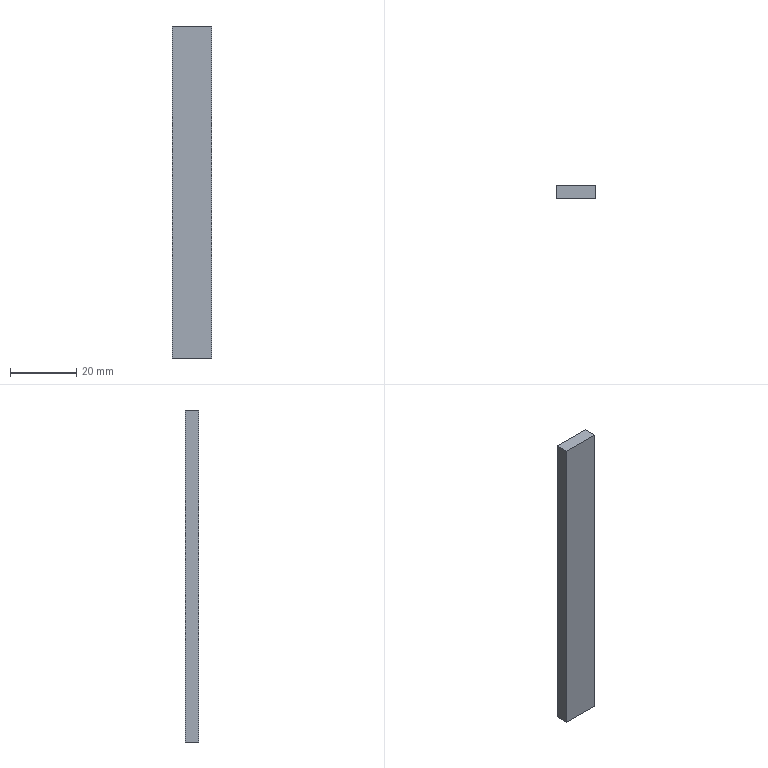Part | STEP file | Guide strip | 1 solid | 6 faces | box 12 x 4 x 100 mm | volume 4800 mm3 | plane 6
STEP:
#1=CARTESIAN_POINT('',(6.,-2.,-50.));
#2=VERTEX_POINT('',#1);
#3=CARTESIAN_POINT('',(6.,2.,-50.));
#4=VERTEX_POINT('',#3);
#5=CARTESIAN_POINT('',(6.,2.,-50.));
#6=DIRECTION('',(0.,1.,0.));
#7=VECTOR('',#6,1000.);
#8=LINE('',#5,#7);
#9=EDGE_CURVE('',#2,#4,#8,.T.);
#10=ORIENTED_EDGE('',*,*,#9,.T.);
#11=CARTESIAN_POINT('',(6.,2.,50.));
#12=VERTEX_POINT('',#11);
#13=CARTESIAN_POINT('',(6.,2.,50.));
#14=DIRECTION('',(0.,0.,-1.));
#15=VECTOR('',#14,1000.);
#16=LINE('',#13,#15);
#17=EDGE_CURVE('',#12,#4,#16,.T.);
#18=ORIENTED_EDGE('',*,*,#17,.F.);
#19=CARTESIAN_POINT('',(6.,-2.,50.));
#20=VERTEX_POINT('',#19);
#21=CARTESIAN_POINT('',(6.,2.,50.));
#22=DIRECTION('',(0.,1.,0.));
#23=VECTOR('',#22,1000.);
#24=LINE('',#21,#23);
#25=EDGE_CURVE('',#20,#12,#24,.T.);
#26=ORIENTED_EDGE('',*,*,#25,.F.);
#27=CARTESIAN_POINT('',(6.,-2.,50.));
#28=DIRECTION('',(0.,0.,-1.));
#29=VECTOR('',#28,1000.);
#30=LINE('',#27,#29);
#31=EDGE_CURVE('',#20,#2,#30,.T.);
#32=ORIENTED_EDGE('',*,*,#31,.T.);
#33=EDGE_LOOP('',(#10,#18,#26,#32));
#34=FACE_OUTER_BOUND('',#33,.T.);
#35=CARTESIAN_POINT('',(6.,2.,50.));
#36=DIRECTION('',(-1.,0.,0.));
#37=DIRECTION('',(0.,0.,1.));
#38=AXIS2_PLACEMENT_3D('',#35,#36,#37);
#39=PLANE('',#38);
#40=ADVANCED_FACE('',(#34),#39,.F.);
#41=CARTESIAN_POINT('',(-6.,2.,-50.));
#42=VERTEX_POINT('',#41);
#43=CARTESIAN_POINT('',(-6.,2.,-50.));
#44=DIRECTION('',(-1.,0.,0.));
#45=VECTOR('',#44,1000.);
#46=LINE('',#43,#45);
#47=EDGE_CURVE('',#4,#42,#46,.T.);
#48=ORIENTED_EDGE('',*,*,#47,.T.);
#49=CARTESIAN_POINT('',(-6.,2.,50.));
#50=VERTEX_POINT('',#49);
#51=CARTESIAN_POINT('',(-6.,2.,50.));
#52=DIRECTION('',(0.,0.,-1.));
#53=VECTOR('',#52,1000.);
#54=LINE('',#51,#53);
#55=EDGE_CURVE('',#50,#42,#54,.T.);
#56=ORIENTED_EDGE('',*,*,#55,.F.);
#57=CARTESIAN_POINT('',(-6.,2.,50.));
#58=DIRECTION('',(-1.,0.,0.));
#59=VECTOR('',#58,1000.);
#60=LINE('',#57,#59);
#61=EDGE_CURVE('',#12,#50,#60,.T.);
#62=ORIENTED_EDGE('',*,*,#61,.F.);
#63=ORIENTED_EDGE('',*,*,#17,.T.);
#64=EDGE_LOOP('',(#48,#56,#62,#63));
#65=FACE_OUTER_BOUND('',#64,.T.);
#66=CARTESIAN_POINT('',(-6.,2.,50.));
#67=DIRECTION('',(0.,-1.,0.));
#68=DIRECTION('',(0.,0.,-1.));
#69=AXIS2_PLACEMENT_3D('',#66,#67,#68);
#70=PLANE('',#69);
#71=ADVANCED_FACE('',(#65),#70,.F.);
#72=CARTESIAN_POINT('',(-6.,-2.,-50.));
#73=VERTEX_POINT('',#72);
#74=CARTESIAN_POINT('',(-6.,2.,-50.));
#75=DIRECTION('',(0.,-1.,0.));
#76=VECTOR('',#75,1000.);
#77=LINE('',#74,#76);
#78=EDGE_CURVE('',#42,#73,#77,.T.);
#79=ORIENTED_EDGE('',*,*,#78,.T.);
#80=CARTESIAN_POINT('',(-6.,-2.,50.));
#81=VERTEX_POINT('',#80);
#82=CARTESIAN_POINT('',(-6.,-2.,50.));
#83=DIRECTION('',(0.,0.,-1.));
#84=VECTOR('',#83,1000.);
#85=LINE('',#82,#84);
#86=EDGE_CURVE('',#81,#73,#85,.T.);
#87=ORIENTED_EDGE('',*,*,#86,.F.);
#88=CARTESIAN_POINT('',(-6.,2.,50.));
#89=DIRECTION('',(0.,-1.,0.));
#90=VECTOR('',#89,1000.);
#91=LINE('',#88,#90);
#92=EDGE_CURVE('',#50,#81,#91,.T.);
#93=ORIENTED_EDGE('',*,*,#92,.F.);
#94=ORIENTED_EDGE('',*,*,#55,.T.);
#95=EDGE_LOOP('',(#79,#87,#93,#94));
#96=FACE_OUTER_BOUND('',#95,.T.);
#97=CARTESIAN_POINT('',(-6.,2.,50.));
#98=DIRECTION('',(1.,0.,0.));
#99=DIRECTION('',(0.,0.,-1.));
#100=AXIS2_PLACEMENT_3D('',#97,#98,#99);
#101=PLANE('',#100);
#102=ADVANCED_FACE('',(#96),#101,.F.);
#103=CARTESIAN_POINT('',(-6.,-2.,-50.));
#104=DIRECTION('',(1.,0.,0.));
#105=VECTOR('',#104,1000.);
#106=LINE('',#103,#105);
#107=EDGE_CURVE('',#73,#2,#106,.T.);
#108=ORIENTED_EDGE('',*,*,#107,.T.);
#109=ORIENTED_EDGE('',*,*,#31,.F.);
#110=CARTESIAN_POINT('',(-6.,-2.,50.));
#111=DIRECTION('',(1.,0.,0.));
#112=VECTOR('',#111,1000.);
#113=LINE('',#110,#112);
#114=EDGE_CURVE('',#81,#20,#113,.T.);
#115=ORIENTED_EDGE('',*,*,#114,.F.);
#116=ORIENTED_EDGE('',*,*,#86,.T.);
#117=EDGE_LOOP('',(#108,#109,#115,#116));
#118=FACE_OUTER_BOUND('',#117,.T.);
#119=CARTESIAN_POINT('',(-6.,-2.,50.));
#120=DIRECTION('',(0.,1.,0.));
#121=DIRECTION('',(0.,0.,1.));
#122=AXIS2_PLACEMENT_3D('',#119,#120,#121);
#123=PLANE('',#122);
#124=ADVANCED_FACE('',(#118),#123,.F.);
#125=ORIENTED_EDGE('',*,*,#25,.T.);
#126=ORIENTED_EDGE('',*,*,#61,.T.);
#127=ORIENTED_EDGE('',*,*,#92,.T.);
#128=ORIENTED_EDGE('',*,*,#114,.T.);
#129=EDGE_LOOP('',(#125,#126,#127,#128));
#130=FACE_OUTER_BOUND('',#129,.T.);
#131=CARTESIAN_POINT('',(0.,0.,50.));
#132=DIRECTION('',(0.,0.,1.));
#133=DIRECTION('',(1.,0.,0.));
#134=AXIS2_PLACEMENT_3D('',#131,#132,#133);
#135=PLANE('',#134);
#136=ADVANCED_FACE('',(#130),#135,.T.);
#137=ORIENTED_EDGE('',*,*,#9,.F.);
#138=ORIENTED_EDGE('',*,*,#107,.F.);
#139=ORIENTED_EDGE('',*,*,#78,.F.);
#140=ORIENTED_EDGE('',*,*,#47,.F.);
#141=EDGE_LOOP('',(#137,#138,#139,#140));
#142=FACE_OUTER_BOUND('',#141,.T.);
#143=CARTESIAN_POINT('',(0.,0.,-50.));
#144=DIRECTION('',(0.,0.,1.));
#145=DIRECTION('',(1.,0.,0.));
#146=AXIS2_PLACEMENT_3D('',#143,#144,#145);
#147=PLANE('',#146);
#148=ADVANCED_FACE('',(#142),#147,.F.);
#149=CLOSED_SHELL('',(#40,#71,#102,#124,#136,#148));
#150=MANIFOLD_SOLID_BREP('',#149);
#151=CARTESIAN_POINT('',(0.,0.,0.));
#152=DIRECTION('',(0.,0.,1.));
#153=DIRECTION('',(1.,0.,0.));
#154=AXIS2_PLACEMENT_3D('',#151,#152,#153);
#155=(LENGTH_UNIT()NAMED_UNIT(*)SI_UNIT(.MILLI.,.METRE.));
#156=UNCERTAINTY_MEASURE_WITH_UNIT(LENGTH_MEASURE(0.00001),#155,'','');
#157=(NAMED_UNIT(*)PLANE_ANGLE_UNIT()SI_UNIT($,.RADIAN.));
#158=(NAMED_UNIT(*)SI_UNIT($,.STERADIAN.)SOLID_ANGLE_UNIT());
#159=(GEOMETRIC_REPRESENTATION_CONTEXT(3)GLOBAL_UNCERTAINTY_ASSIGNED_CONTEXT((#156))GLOBAL_UNIT_ASSIGNED_CONTEXT((#155,#157,#158))REPRESENTATION_CONTEXT('',''));
#160=ADVANCED_BREP_SHAPE_REPRESENTATION('',(#150,#154),#159);